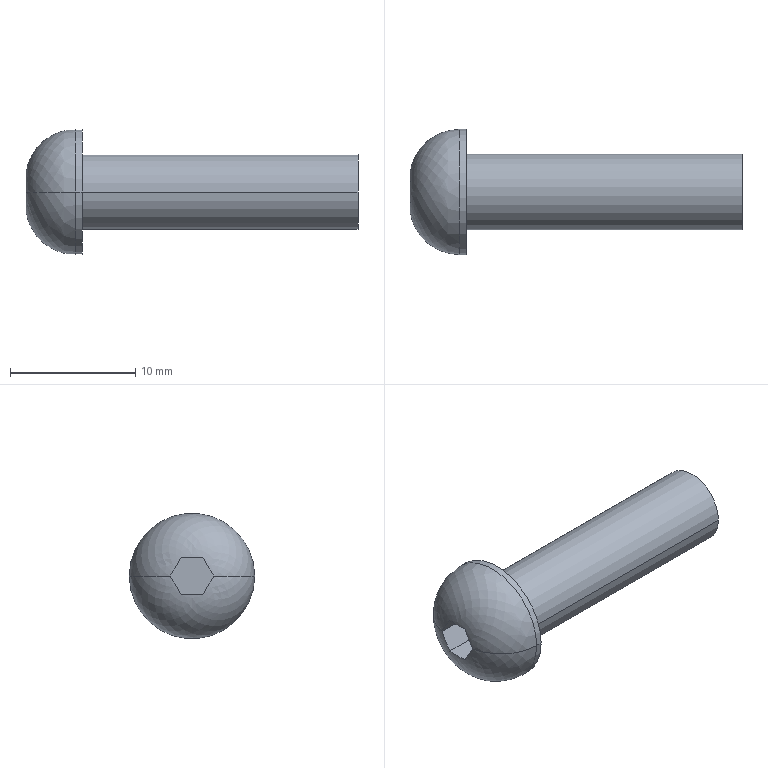Part | STEP file | Standoff screw φ6x12(M5) | 1 solid | 15 faces | box 26.469 x 10 x 10 mm | volume 868.238 mm3 | plane 9 | cylinder 4 | other 2 | commonest cylinder face diameters 6 x2 10 x2
STEP:
#1=CARTESIAN_POINT('',(0.,0.,0.));
#2=DIRECTION('',(0.,0.,1.));
#3=DIRECTION('',(1.,0.,0.));
#4=AXIS2_PLACEMENT_3D('',#1,#2,#3);
#5=CARTESIAN_POINT('',(4.5,3.,0.));
#6=VERTEX_POINT('',#5);
#7=CARTESIAN_POINT('',(4.5,-3.,0.));
#8=VERTEX_POINT('',#7);
#9=CARTESIAN_POINT('',(4.5,0.,0.));
#10=DIRECTION('',(1.,0.,0.));
#11=DIRECTION('',(0.,1.,0.));
#12=AXIS2_PLACEMENT_3D('',#9,#10,#11);
#13=CIRCLE('',#12,3.);
#14=CARTESIAN_POINT('',(26.5,0.,0.));
#15=DIRECTION('',(1.,0.,0.));
#16=DIRECTION('',(0.,1.,0.));
#17=AXIS2_PLACEMENT_3D('',#14,#15,#16);
#18=CYLINDRICAL_SURFACE('',#17,3.);
#19=CARTESIAN_POINT('',(0.,-22.));
#20=DIRECTION('',(1.,0.));
#21=VECTOR('',#20,1.);
#22=LINE('',#19,#21);
#23=(GEOMETRIC_REPRESENTATION_CONTEXT(2)PARAMETRIC_REPRESENTATION_CONTEXT()REPRESENTATION_CONTEXT('',''));
#24=DEFINITIONAL_REPRESENTATION('',(#22),#23);
#25=PCURVE('',#18,#24);
#26=CARTESIAN_POINT('',(4.5,-5.,0.));
#27=DIRECTION('',(-1.,0.,0.));
#28=DIRECTION('',(0.,-1.,0.));
#29=AXIS2_PLACEMENT_3D('',#26,#27,#28);
#30=PLANE('',#29);
#31=CARTESIAN_POINT('',(-8.,0.));
#32=CARTESIAN_POINT('',(-8.,5.196));
#33=CARTESIAN_POINT('',(-3.5,2.598));
#34=CARTESIAN_POINT('',(1.,0.));
#35=CARTESIAN_POINT('',(-3.5,-2.598));
#36=CARTESIAN_POINT('',(-8.,-5.196));
#37=CARTESIAN_POINT('',(-8.,0.));
#38=(BOUNDED_CURVE()B_SPLINE_CURVE(2,(#31,#32,#33,#34,#35,#36,#37),.UNSPECIFIED.,.T.,.F.)B_SPLINE_CURVE_WITH_KNOTS((1,2,2,2,2,1),(-2.094,0.,2.094,4.189,6.283,8.378),.UNSPECIFIED.)CURVE()GEOMETRIC_REPRESENTATION_ITEM()RATIONAL_B_SPLINE_CURVE((1.,0.5,1.,0.5,1.,0.5,1.))REPRESENTATION_ITEM(''));
#39=(GEOMETRIC_REPRESENTATION_CONTEXT(2)PARAMETRIC_REPRESENTATION_CONTEXT()REPRESENTATION_CONTEXT('',''));
#40=DEFINITIONAL_REPRESENTATION('',(#38),#39);
#41=PCURVE('',#30,#40);
#42=SURFACE_CURVE('',#13,(#25,#41),.PCURVE_S1.);
#43=EDGE_CURVE('',#6,#8,#42,.T.);
#44=ORIENTED_EDGE('',*,*,#43,.T.);
#45=CARTESIAN_POINT('',(26.5,-3.,0.));
#46=VERTEX_POINT('',#45);
#47=CARTESIAN_POINT('',(26.5,-3.,0.));
#48=DIRECTION('',(1.,0.,0.));
#49=VECTOR('',#48,1.);
#50=LINE('',#47,#49);
#51=CARTESIAN_POINT('',(3.142,0.));
#52=DIRECTION('',(0.,1.));
#53=VECTOR('',#52,1.);
#54=LINE('',#51,#53);
#55=(GEOMETRIC_REPRESENTATION_CONTEXT(2)PARAMETRIC_REPRESENTATION_CONTEXT()REPRESENTATION_CONTEXT('',''));
#56=DEFINITIONAL_REPRESENTATION('',(#54),#55);
#57=PCURVE('',#18,#56);
#58=CARTESIAN_POINT('',(26.5,0.,0.));
#59=DIRECTION('',(1.,0.,0.));
#60=DIRECTION('',(0.,1.,0.));
#61=AXIS2_PLACEMENT_3D('',#58,#59,#60);
#62=CYLINDRICAL_SURFACE('',#61,3.);
#63=CARTESIAN_POINT('',(3.142,0.));
#64=DIRECTION('',(0.,1.));
#65=VECTOR('',#64,1.);
#66=LINE('',#63,#65);
#67=(GEOMETRIC_REPRESENTATION_CONTEXT(2)PARAMETRIC_REPRESENTATION_CONTEXT()REPRESENTATION_CONTEXT('',''));
#68=DEFINITIONAL_REPRESENTATION('',(#66),#67);
#69=PCURVE('',#62,#68);
#70=SURFACE_CURVE('',#50,(#57,#69),.PCURVE_S1.);
#71=EDGE_CURVE('',#8,#46,#70,.T.);
#72=ORIENTED_EDGE('',*,*,#71,.T.);
#73=CARTESIAN_POINT('',(26.5,3.,0.));
#74=VERTEX_POINT('',#73);
#75=CARTESIAN_POINT('',(26.5,0.,0.));
#76=DIRECTION('',(1.,0.,0.));
#77=DIRECTION('',(0.,1.,0.));
#78=AXIS2_PLACEMENT_3D('',#75,#76,#77);
#79=CIRCLE('',#78,3.);
#80=CARTESIAN_POINT('',(0.,0.));
#81=DIRECTION('',(1.,0.));
#82=VECTOR('',#81,1.);
#83=LINE('',#80,#82);
#84=(GEOMETRIC_REPRESENTATION_CONTEXT(2)PARAMETRIC_REPRESENTATION_CONTEXT()REPRESENTATION_CONTEXT('',''));
#85=DEFINITIONAL_REPRESENTATION('',(#83),#84);
#86=PCURVE('',#18,#85);
#87=CARTESIAN_POINT('',(26.5,-3.,0.));
#88=DIRECTION('',(-1.,0.,0.));
#89=DIRECTION('',(0.,-1.,0.));
#90=AXIS2_PLACEMENT_3D('',#87,#88,#89);
#91=PLANE('',#90);
#92=CARTESIAN_POINT('',(-6.,0.));
#93=CARTESIAN_POINT('',(-6.,5.196));
#94=CARTESIAN_POINT('',(-1.5,2.598));
#95=CARTESIAN_POINT('',(3.,0.));
#96=CARTESIAN_POINT('',(-1.5,-2.598));
#97=CARTESIAN_POINT('',(-6.,-5.196));
#98=CARTESIAN_POINT('',(-6.,0.));
#99=(BOUNDED_CURVE()B_SPLINE_CURVE(2,(#92,#93,#94,#95,#96,#97,#98),.UNSPECIFIED.,.T.,.F.)B_SPLINE_CURVE_WITH_KNOTS((1,2,2,2,2,1),(-2.094,0.,2.094,4.189,6.283,8.378),.UNSPECIFIED.)CURVE()GEOMETRIC_REPRESENTATION_ITEM()RATIONAL_B_SPLINE_CURVE((1.,0.5,1.,0.5,1.,0.5,1.))REPRESENTATION_ITEM(''));
#100=(GEOMETRIC_REPRESENTATION_CONTEXT(2)PARAMETRIC_REPRESENTATION_CONTEXT()REPRESENTATION_CONTEXT('',''));
#101=DEFINITIONAL_REPRESENTATION('',(#99),#100);
#102=PCURVE('',#91,#101);
#103=SURFACE_CURVE('',#79,(#86,#102),.PCURVE_S1.);
#104=EDGE_CURVE('',#74,#46,#103,.T.);
#105=ORIENTED_EDGE('',*,*,#104,.F.);
#106=CARTESIAN_POINT('',(26.5,3.,0.));
#107=DIRECTION('',(1.,0.,0.));
#108=VECTOR('',#107,1.);
#109=LINE('',#106,#108);
#110=CARTESIAN_POINT('',(0.,0.));
#111=DIRECTION('',(0.,1.));
#112=VECTOR('',#111,1.);
#113=LINE('',#110,#112);
#114=(GEOMETRIC_REPRESENTATION_CONTEXT(2)PARAMETRIC_REPRESENTATION_CONTEXT()REPRESENTATION_CONTEXT('',''));
#115=DEFINITIONAL_REPRESENTATION('',(#113),#114);
#116=PCURVE('',#18,#115);
#117=CARTESIAN_POINT('',(6.283,0.));
#118=DIRECTION('',(0.,1.));
#119=VECTOR('',#118,1.);
#120=LINE('',#117,#119);
#121=(GEOMETRIC_REPRESENTATION_CONTEXT(2)PARAMETRIC_REPRESENTATION_CONTEXT()REPRESENTATION_CONTEXT('',''));
#122=DEFINITIONAL_REPRESENTATION('',(#120),#121);
#123=PCURVE('',#62,#122);
#124=SURFACE_CURVE('',#109,(#116,#123),.PCURVE_S1.);
#125=EDGE_CURVE('',#6,#74,#124,.T.);
#126=ORIENTED_EDGE('',*,*,#125,.F.);
#127=EDGE_LOOP('',(#44,#72,#105,#126));
#128=FACE_BOUND('',#127,.T.);
#129=ADVANCED_FACE('',(#128),#18,.T.);
#130=CARTESIAN_POINT('',(4.,5.,0.));
#131=VERTEX_POINT('',#130);
#132=CARTESIAN_POINT('',(4.,-5.,0.));
#133=VERTEX_POINT('',#132);
#134=CARTESIAN_POINT('',(4.,0.,0.));
#135=DIRECTION('',(1.,0.,0.));
#136=DIRECTION('',(0.,1.,0.));
#137=AXIS2_PLACEMENT_3D('',#134,#135,#136);
#138=CIRCLE('',#137,5.);
#139=CARTESIAN_POINT('',(26.5,0.,0.));
#140=DIRECTION('',(1.,0.,0.));
#141=DIRECTION('',(0.,1.,0.));
#142=AXIS2_PLACEMENT_3D('',#139,#140,#141);
#143=CYLINDRICAL_SURFACE('',#142,5.);
#144=CARTESIAN_POINT('',(0.,-22.5));
#145=DIRECTION('',(1.,0.));
#146=VECTOR('',#145,1.);
#147=LINE('',#144,#146);
#148=(GEOMETRIC_REPRESENTATION_CONTEXT(2)PARAMETRIC_REPRESENTATION_CONTEXT()REPRESENTATION_CONTEXT('',''));
#149=DEFINITIONAL_REPRESENTATION('',(#147),#148);
#150=PCURVE('',#143,#149);
#151=CARTESIAN_POINT('',(0.03137,1.5,0.));
#152=CARTESIAN_POINT('',(0.0916,1.978,0.));
#153=CARTESIAN_POINT('',(0.2209,2.447,0.));
#154=CARTESIAN_POINT('',(0.4178,2.896,0.));
#155=CARTESIAN_POINT('',(0.6776,3.31,0.));
#156=CARTESIAN_POINT('',(0.9929,3.681,0.));
#157=CARTESIAN_POINT('',(1.716,4.319,0.));
#158=CARTESIAN_POINT('',(2.123,4.585,0.));
#159=CARTESIAN_POINT('',(2.567,4.791,0.));
#160=CARTESIAN_POINT('',(3.036,4.93,0.));
#161=CARTESIAN_POINT('',(3.518,5.,0.));
#162=CARTESIAN_POINT('',(4.,5.,0.));
#163=B_SPLINE_CURVE_WITH_KNOTS('',6,(#151,#152,#153,#154,#155,#156,#157,#158,#159,#160,#161,#162),.UNSPECIFIED.,.F.,.F.,(7,5,7),(4.838,5.56,6.283),.UNSPECIFIED.);
#164=CARTESIAN_POINT('',(4.,0.,0.));
#165=DIRECTION('',(1.,0.,0.));
#166=AXIS1_PLACEMENT('',#164,#165);
#167=SURFACE_OF_REVOLUTION('',#163,#166);
#168=CARTESIAN_POINT('',(0.,6.283));
#169=DIRECTION('',(1.,0.));
#170=VECTOR('',#169,1.);
#171=LINE('',#168,#170);
#172=(GEOMETRIC_REPRESENTATION_CONTEXT(2)PARAMETRIC_REPRESENTATION_CONTEXT()REPRESENTATION_CONTEXT('',''));
#173=DEFINITIONAL_REPRESENTATION('',(#171),#172);
#174=PCURVE('',#167,#173);
#175=SURFACE_CURVE('',#138,(#150,#174),.PCURVE_S1.);
#176=EDGE_CURVE('',#131,#133,#175,.T.);
#177=ORIENTED_EDGE('',*,*,#176,.T.);
#178=CARTESIAN_POINT('',(4.5,-5.,0.));
#179=VERTEX_POINT('',#178);
#180=CARTESIAN_POINT('',(26.5,-5.,0.));
#181=DIRECTION('',(1.,0.,0.));
#182=VECTOR('',#181,1.);
#183=LINE('',#180,#182);
#184=CARTESIAN_POINT('',(3.142,0.));
#185=DIRECTION('',(0.,1.));
#186=VECTOR('',#185,1.);
#187=LINE('',#184,#186);
#188=(GEOMETRIC_REPRESENTATION_CONTEXT(2)PARAMETRIC_REPRESENTATION_CONTEXT()REPRESENTATION_CONTEXT('',''));
#189=DEFINITIONAL_REPRESENTATION('',(#187),#188);
#190=PCURVE('',#143,#189);
#191=CARTESIAN_POINT('',(26.5,0.,0.));
#192=DIRECTION('',(1.,0.,0.));
#193=DIRECTION('',(0.,1.,0.));
#194=AXIS2_PLACEMENT_3D('',#191,#192,#193);
#195=CYLINDRICAL_SURFACE('',#194,5.);
#196=CARTESIAN_POINT('',(3.142,0.));
#197=DIRECTION('',(0.,1.));
#198=VECTOR('',#197,1.);
#199=LINE('',#196,#198);
#200=(GEOMETRIC_REPRESENTATION_CONTEXT(2)PARAMETRIC_REPRESENTATION_CONTEXT()REPRESENTATION_CONTEXT('',''));
#201=DEFINITIONAL_REPRESENTATION('',(#199),#200);
#202=PCURVE('',#195,#201);
#203=SURFACE_CURVE('',#183,(#190,#202),.PCURVE_S1.);
#204=EDGE_CURVE('',#133,#179,#203,.T.);
#205=ORIENTED_EDGE('',*,*,#204,.T.);
#206=CARTESIAN_POINT('',(4.5,5.,0.));
#207=VERTEX_POINT('',#206);
#208=CARTESIAN_POINT('',(4.5,0.,0.));
#209=DIRECTION('',(1.,0.,0.));
#210=DIRECTION('',(0.,1.,0.));
#211=AXIS2_PLACEMENT_3D('',#208,#209,#210);
#212=CIRCLE('',#211,5.);
#213=CARTESIAN_POINT('',(0.,-22.));
#214=DIRECTION('',(1.,0.));
#215=VECTOR('',#214,1.);
#216=LINE('',#213,#215);
#217=(GEOMETRIC_REPRESENTATION_CONTEXT(2)PARAMETRIC_REPRESENTATION_CONTEXT()REPRESENTATION_CONTEXT('',''));
#218=DEFINITIONAL_REPRESENTATION('',(#216),#217);
#219=PCURVE('',#143,#218);
#220=CARTESIAN_POINT('',(-10.,0.));
#221=CARTESIAN_POINT('',(-10.,8.66));
#222=CARTESIAN_POINT('',(-2.5,4.33));
#223=CARTESIAN_POINT('',(5.,0.));
#224=CARTESIAN_POINT('',(-2.5,-4.33));
#225=CARTESIAN_POINT('',(-10.,-8.66));
#226=CARTESIAN_POINT('',(-10.,0.));
#227=(BOUNDED_CURVE()B_SPLINE_CURVE(2,(#220,#221,#222,#223,#224,#225,#226),.UNSPECIFIED.,.T.,.F.)B_SPLINE_CURVE_WITH_KNOTS((1,2,2,2,2,1),(-2.094,0.,2.094,4.189,6.283,8.378),.UNSPECIFIED.)CURVE()GEOMETRIC_REPRESENTATION_ITEM()RATIONAL_B_SPLINE_CURVE((1.,0.5,1.,0.5,1.,0.5,1.))REPRESENTATION_ITEM(''));
#228=(GEOMETRIC_REPRESENTATION_CONTEXT(2)PARAMETRIC_REPRESENTATION_CONTEXT()REPRESENTATION_CONTEXT('',''));
#229=DEFINITIONAL_REPRESENTATION('',(#227),#228);
#230=PCURVE('',#30,#229);
#231=SURFACE_CURVE('',#212,(#219,#230),.PCURVE_S1.);
#232=EDGE_CURVE('',#207,#179,#231,.T.);
#233=ORIENTED_EDGE('',*,*,#232,.F.);
#234=CARTESIAN_POINT('',(26.5,5.,0.));
#235=DIRECTION('',(1.,0.,0.));
#236=VECTOR('',#235,1.);
#237=LINE('',#234,#236);
#238=CARTESIAN_POINT('',(0.,0.));
#239=DIRECTION('',(0.,1.));
#240=VECTOR('',#239,1.);
#241=LINE('',#238,#240);
#242=(GEOMETRIC_REPRESENTATION_CONTEXT(2)PARAMETRIC_REPRESENTATION_CONTEXT()REPRESENTATION_CONTEXT('',''));
#243=DEFINITIONAL_REPRESENTATION('',(#241),#242);
#244=PCURVE('',#143,#243);
#245=CARTESIAN_POINT('',(6.283,0.));
#246=DIRECTION('',(0.,1.));
#247=VECTOR('',#246,1.);
#248=LINE('',#245,#247);
#249=(GEOMETRIC_REPRESENTATION_CONTEXT(2)PARAMETRIC_REPRESENTATION_CONTEXT()REPRESENTATION_CONTEXT('',''));
#250=DEFINITIONAL_REPRESENTATION('',(#248),#249);
#251=PCURVE('',#195,#250);
#252=SURFACE_CURVE('',#237,(#244,#251),.PCURVE_S1.);
#253=EDGE_CURVE('',#131,#207,#252,.T.);
#254=ORIENTED_EDGE('',*,*,#253,.F.);
#255=EDGE_LOOP('',(#177,#205,#233,#254));
#256=FACE_BOUND('',#255,.T.);
#257=ADVANCED_FACE('',(#256),#143,.T.);
#258=CARTESIAN_POINT('',(0.06756,-0.866,1.5));
#259=VERTEX_POINT('',#258);
#260=CARTESIAN_POINT('',(0.06756,-1.732,0.));
#261=VERTEX_POINT('',#260);
#262=CARTESIAN_POINT('',(0.06756,-0.866,1.5));
#263=CARTESIAN_POINT('',(0.04069,-1.01,1.25));
#264=CARTESIAN_POINT('',(0.02206,-1.299,0.75));
#265=CARTESIAN_POINT('',(0.04069,-1.588,0.25));
#266=CARTESIAN_POINT('',(0.06756,-1.732,0.));
#267=B_SPLINE_CURVE_WITH_KNOTS('',3,(#262,#263,#264,#265,#266),.UNSPECIFIED.,.F.,.F.,(4,1,4),(0.000000231,0.0008663,0.001732),.UNSPECIFIED.);
#268=CARTESIAN_POINT('',(2.094,4.896));
#269=CARTESIAN_POINT('',(2.108,4.893));
#270=CARTESIAN_POINT('',(2.134,4.887));
#271=CARTESIAN_POINT('',(2.176,4.878));
#272=CARTESIAN_POINT('',(2.22,4.87));
#273=CARTESIAN_POINT('',(2.266,4.862));
#274=CARTESIAN_POINT('',(2.313,4.856));
#275=CARTESIAN_POINT('',(2.361,4.85));
#276=CARTESIAN_POINT('',(2.411,4.846));
#277=CARTESIAN_POINT('',(2.462,4.842));
#278=CARTESIAN_POINT('',(2.513,4.84));
#279=CARTESIAN_POINT('',(2.566,4.838));
#280=CARTESIAN_POINT('',(2.618,4.838));
#281=CARTESIAN_POINT('',(2.67,4.838));
#282=CARTESIAN_POINT('',(2.723,4.84));
#283=CARTESIAN_POINT('',(2.774,4.842));
#284=CARTESIAN_POINT('',(2.825,4.846));
#285=CARTESIAN_POINT('',(2.875,4.85));
#286=CARTESIAN_POINT('',(2.923,4.856));
#287=CARTESIAN_POINT('',(2.97,4.862));
#288=CARTESIAN_POINT('',(3.016,4.87));
#289=CARTESIAN_POINT('',(3.06,4.878));
#290=CARTESIAN_POINT('',(3.102,4.887));
#291=CARTESIAN_POINT('',(3.128,4.893));
#292=CARTESIAN_POINT('',(3.142,4.896));
#293=B_SPLINE_CURVE_WITH_KNOTS('',3,(#268,#269,#270,#271,#272,#273,#274,#275,#276,#277,#278,#279,#280,#281,#282,#283,#284,#285,#286,#287,#288,#289,#290,#291,#292),.UNSPECIFIED.,.F.,.F.,(4,1,1,1,1,1,1,1,1,1,1,1,1,1,1,1,1,1,1,1,1,1,4),(0.000000231,0.00007896,0.0001577,0.0002364,0.0003151,0.0003939,0.0004726,0.0005513,0.0006301,0.0007088,0.0007875,0.0008663,0.000945,0.001024,0.001102,0.001181,0.00126,0.001339,0.001417,0.001496,0.001575,0.001654,0.001732),.QUASI_UNIFORM_KNOTS.);
#294=(GEOMETRIC_REPRESENTATION_CONTEXT(2)PARAMETRIC_REPRESENTATION_CONTEXT()REPRESENTATION_CONTEXT('',''));
#295=DEFINITIONAL_REPRESENTATION('',(#293),#294);
#296=PCURVE('',#167,#295);
#297=CARTESIAN_POINT('',(2.4,-1.732,0.));
#298=DIRECTION('',(0.,-0.866,0.5));
#299=DIRECTION('',(0.,-0.5,-0.866));
#300=AXIS2_PLACEMENT_3D('',#297,#298,#299);
#301=PLANE('',#300);
#302=CARTESIAN_POINT('',(-1.732,-2.332));
#303=CARTESIAN_POINT('',(-1.443,-2.359));
#304=CARTESIAN_POINT('',(-0.866,-2.378));
#305=CARTESIAN_POINT('',(-0.2887,-2.359));
#306=CARTESIAN_POINT('',(0.,-2.332));
#307=B_SPLINE_CURVE_WITH_KNOTS('',3,(#302,#303,#304,#305,#306),.UNSPECIFIED.,.F.,.F.,(4,1,4),(0.000000231,0.0008663,0.001732),.UNSPECIFIED.);
#308=(GEOMETRIC_REPRESENTATION_CONTEXT(2)PARAMETRIC_REPRESENTATION_CONTEXT()REPRESENTATION_CONTEXT('',''));
#309=DEFINITIONAL_REPRESENTATION('',(#307),#308);
#310=PCURVE('',#301,#309);
#311=SURFACE_CURVE('',#267,(#296,#310),.PCURVE_S1.);
#312=EDGE_CURVE('',#259,#261,#311,.T.);
#313=ORIENTED_EDGE('',*,*,#312,.T.);
#314=CARTESIAN_POINT('',(4.,-1.,0.));
#315=DIRECTION('',(0.,0.,1.));
#316=DIRECTION('',(0.,-1.,0.));
#317=AXIS2_PLACEMENT_3D('',#314,#315,#316);
#318=CIRCLE('',#317,4.);
#319=CARTESIAN_POINT('',(3.142,0.));
#320=DIRECTION('',(0.,1.));
#321=VECTOR('',#320,1.);
#322=LINE('',#319,#321);
#323=(GEOMETRIC_REPRESENTATION_CONTEXT(2)PARAMETRIC_REPRESENTATION_CONTEXT()REPRESENTATION_CONTEXT('',''));
#324=DEFINITIONAL_REPRESENTATION('',(#322),#323);
#325=PCURVE('',#167,#324);
#326=CARTESIAN_POINT('',(0.03137,1.5,0.));
#327=CARTESIAN_POINT('',(0.0916,1.978,0.));
#328=CARTESIAN_POINT('',(0.2209,2.447,0.));
#329=CARTESIAN_POINT('',(0.4178,2.896,0.));
#330=CARTESIAN_POINT('',(0.6776,3.31,0.));
#331=CARTESIAN_POINT('',(0.9929,3.681,0.));
#332=CARTESIAN_POINT('',(1.716,4.319,0.));
#333=CARTESIAN_POINT('',(2.123,4.585,0.));
#334=CARTESIAN_POINT('',(2.567,4.791,0.));
#335=CARTESIAN_POINT('',(3.036,4.93,0.));
#336=CARTESIAN_POINT('',(3.518,5.,0.));
#337=CARTESIAN_POINT('',(4.,5.,0.));
#338=B_SPLINE_CURVE_WITH_KNOTS('',6,(#326,#327,#328,#329,#330,#331,#332,#333,#334,#335,#336,#337),.UNSPECIFIED.,.F.,.F.,(7,5,7),(4.838,5.56,6.283),.UNSPECIFIED.);
#339=CARTESIAN_POINT('',(4.,0.,0.));
#340=DIRECTION('',(1.,0.,0.));
#341=AXIS1_PLACEMENT('',#339,#340);
#342=SURFACE_OF_REVOLUTION('',#338,#341);
#343=CARTESIAN_POINT('',(3.142,0.));
#344=DIRECTION('',(0.,1.));
#345=VECTOR('',#344,1.);
#346=LINE('',#343,#345);
#347=(GEOMETRIC_REPRESENTATION_CONTEXT(2)PARAMETRIC_REPRESENTATION_CONTEXT()REPRESENTATION_CONTEXT('',''));
#348=DEFINITIONAL_REPRESENTATION('',(#346),#347);
#349=PCURVE('',#342,#348);
#350=SURFACE_CURVE('',#318,(#325,#349),.PCURVE_S1.);
#351=EDGE_CURVE('',#261,#133,#350,.T.);
#352=ORIENTED_EDGE('',*,*,#351,.T.);
#353=ORIENTED_EDGE('',*,*,#176,.F.);
#354=CARTESIAN_POINT('',(0.06756,1.732,0.));
#355=VERTEX_POINT('',#354);
#356=CARTESIAN_POINT('',(4.,1.,0.));
#357=DIRECTION('',(0.,0.,-1.));
#358=DIRECTION('',(-1.,0.,0.));
#359=AXIS2_PLACEMENT_3D('',#356,#357,#358);
#360=CIRCLE('',#359,4.);
#361=CARTESIAN_POINT('',(0.,4.712));
#362=DIRECTION('',(0.,1.));
#363=VECTOR('',#362,1.);
#364=LINE('',#361,#363);
#365=(GEOMETRIC_REPRESENTATION_CONTEXT(2)PARAMETRIC_REPRESENTATION_CONTEXT()REPRESENTATION_CONTEXT('',''));
#366=DEFINITIONAL_REPRESENTATION('',(#364),#365);
#367=PCURVE('',#167,#366);
#368=CARTESIAN_POINT('',(6.283,4.712));
#369=DIRECTION('',(0.,1.));
#370=VECTOR('',#369,1.);
#371=LINE('',#368,#370);
#372=(GEOMETRIC_REPRESENTATION_CONTEXT(2)PARAMETRIC_REPRESENTATION_CONTEXT()REPRESENTATION_CONTEXT('',''));
#373=DEFINITIONAL_REPRESENTATION('',(#371),#372);
#374=PCURVE('',#342,#373);
#375=SURFACE_CURVE('',#360,(#367,#374),.PCURVE_S1.);
#376=EDGE_CURVE('',#355,#131,#375,.T.);
#377=ORIENTED_EDGE('',*,*,#376,.F.);
#378=CARTESIAN_POINT('',(0.06756,0.866,1.5));
#379=VERTEX_POINT('',#378);
#380=CARTESIAN_POINT('',(0.06756,1.732,0.));
#381=CARTESIAN_POINT('',(0.04069,1.588,0.25));
#382=CARTESIAN_POINT('',(0.02206,1.299,0.75));
#383=CARTESIAN_POINT('',(0.04069,1.01,1.25));
#384=CARTESIAN_POINT('',(0.06756,0.866,1.5));
#385=B_SPLINE_CURVE_WITH_KNOTS('',3,(#380,#381,#382,#383,#384),.UNSPECIFIED.,.F.,.F.,(4,1,4),(0.000000231,0.0008663,0.001732),.QUASI_UNIFORM_KNOTS.);
#386=CARTESIAN_POINT('',(0.,4.896));
#387=CARTESIAN_POINT('',(0.01312,4.893));
#388=CARTESIAN_POINT('',(0.03996,4.887));
#389=CARTESIAN_POINT('',(0.082,4.878));
#390=CARTESIAN_POINT('',(0.1258,4.87));
#391=CARTESIAN_POINT('',(0.1712,4.862));
#392=CARTESIAN_POINT('',(0.2183,4.856));
#393=CARTESIAN_POINT('',(0.2667,4.85));
#394=CARTESIAN_POINT('',(0.3165,4.846));
#395=CARTESIAN_POINT('',(0.3673,4.842));
#396=CARTESIAN_POINT('',(0.4189,4.84));
#397=CARTESIAN_POINT('',(0.4711,4.838));
#398=CARTESIAN_POINT('',(0.5236,4.838));
#399=CARTESIAN_POINT('',(0.5761,4.838));
#400=CARTESIAN_POINT('',(0.6283,4.84));
#401=CARTESIAN_POINT('',(0.6799,4.842));
#402=CARTESIAN_POINT('',(0.7307,4.846));
#403=CARTESIAN_POINT('',(0.7805,4.85));
#404=CARTESIAN_POINT('',(0.8289,4.856));
#405=CARTESIAN_POINT('',(0.876,4.862));
#406=CARTESIAN_POINT('',(0.9214,4.87));
#407=CARTESIAN_POINT('',(0.9652,4.878));
#408=CARTESIAN_POINT('',(1.007,4.887));
#409=CARTESIAN_POINT('',(1.034,4.893));
#410=CARTESIAN_POINT('',(1.047,4.896));
#411=B_SPLINE_CURVE_WITH_KNOTS('',3,(#386,#387,#388,#389,#390,#391,#392,#393,#394,#395,#396,#397,#398,#399,#400,#401,#402,#403,#404,#405,#406,#407,#408,#409,#410),.UNSPECIFIED.,.F.,.F.,(4,1,1,1,1,1,1,1,1,1,1,1,1,1,1,1,1,1,1,1,1,1,4),(0.000000231,0.00007896,0.0001577,0.0002364,0.0003151,0.0003939,0.0004726,0.0005513,0.0006301,0.0007088,0.0007875,0.0008663,0.000945,0.001024,0.001102,0.001181,0.00126,0.001339,0.001417,0.001496,0.001575,0.001654,0.001732),.QUASI_UNIFORM_KNOTS.);
#412=(GEOMETRIC_REPRESENTATION_CONTEXT(2)PARAMETRIC_REPRESENTATION_CONTEXT()REPRESENTATION_CONTEXT('',''));
#413=DEFINITIONAL_REPRESENTATION('',(#411),#412);
#414=PCURVE('',#167,#413);
#415=CARTESIAN_POINT('',(2.4,0.866,1.5));
#416=DIRECTION('',(0.,0.866,0.5));
#417=DIRECTION('',(0.,-0.5,0.866));
#418=AXIS2_PLACEMENT_3D('',#415,#416,#417);
#419=PLANE('',#418);
#420=CARTESIAN_POINT('',(-1.732,-2.332));
#421=CARTESIAN_POINT('',(-1.443,-2.359));
#422=CARTESIAN_POINT('',(-0.866,-2.378));
#423=CARTESIAN_POINT('',(-0.2887,-2.359));
#424=CARTESIAN_POINT('',(0.,-2.332));
#425=B_SPLINE_CURVE_WITH_KNOTS('',3,(#420,#421,#422,#423,#424),.UNSPECIFIED.,.F.,.F.,(4,1,4),(0.000000231,0.0008663,0.001732),.QUASI_UNIFORM_KNOTS.);
#426=(GEOMETRIC_REPRESENTATION_CONTEXT(2)PARAMETRIC_REPRESENTATION_CONTEXT()REPRESENTATION_CONTEXT('',''));
#427=DEFINITIONAL_REPRESENTATION('',(#425),#426);
#428=PCURVE('',#419,#427);
#429=SURFACE_CURVE('',#385,(#414,#428),.PCURVE_S1.);
#430=EDGE_CURVE('',#355,#379,#429,.T.);
#431=ORIENTED_EDGE('',*,*,#430,.T.);
#432=CARTESIAN_POINT('',(0.06756,0.866,1.5));
#433=CARTESIAN_POINT('',(0.04093,0.5799,1.5));
#434=CARTESIAN_POINT('',(0.0314,0.2903,1.5));
#435=CARTESIAN_POINT('',(0.03134,-0.2878,1.5));
#436=CARTESIAN_POINT('',(0.04077,-0.5782,1.5));
#437=CARTESIAN_POINT('',(0.06756,-0.866,1.5));
#438=B_SPLINE_CURVE_WITH_KNOTS('',3,(#432,#433,#434,#435,#436,#437),.UNSPECIFIED.,.F.,.F.,(4,2,4),(0.0271,0.02797,0.02884),.UNSPECIFIED.);
#439=CARTESIAN_POINT('',(1.047,4.896));
#440=CARTESIAN_POINT('',(1.06,4.893));
#441=CARTESIAN_POINT('',(1.087,4.887));
#442=CARTESIAN_POINT('',(1.129,4.878));
#443=CARTESIAN_POINT('',(1.172,4.87));
#444=CARTESIAN_POINT('',(1.217,4.862));
#445=CARTESIAN_POINT('',(1.264,4.856));
#446=CARTESIAN_POINT('',(1.313,4.85));
#447=CARTESIAN_POINT('',(1.363,4.846));
#448=CARTESIAN_POINT('',(1.413,4.842));
#449=CARTESIAN_POINT('',(1.465,4.84));
#450=CARTESIAN_POINT('',(1.517,4.838));
#451=CARTESIAN_POINT('',(1.57,4.838));
#452=CARTESIAN_POINT('',(1.623,4.838));
#453=CARTESIAN_POINT('',(1.675,4.84));
#454=CARTESIAN_POINT('',(1.727,4.842));
#455=CARTESIAN_POINT('',(1.778,4.846));
#456=CARTESIAN_POINT('',(1.827,4.85));
#457=CARTESIAN_POINT('',(1.876,4.856));
#458=CARTESIAN_POINT('',(1.923,4.862));
#459=CARTESIAN_POINT('',(1.969,4.87));
#460=CARTESIAN_POINT('',(2.013,4.878));
#461=CARTESIAN_POINT('',(2.055,4.887));
#462=CARTESIAN_POINT('',(2.081,4.893));
#463=CARTESIAN_POINT('',(2.094,4.896));
#464=B_SPLINE_CURVE_WITH_KNOTS('',3,(#439,#440,#441,#442,#443,#444,#445,#446,#447,#448,#449,#450,#451,#452,#453,#454,#455,#456,#457,#458,#459,#460,#461,#462,#463),.UNSPECIFIED.,.F.,.F.,(4,1,1,1,1,1,1,1,1,1,1,1,1,1,1,1,1,1,1,1,1,1,4),(0.0271,0.02718,0.02726,0.02734,0.02742,0.0275,0.02758,0.02765,0.02773,0.02781,0.02789,0.02797,0.02805,0.02813,0.02821,0.02828,0.02836,0.02844,0.02852,0.0286,0.02868,0.02876,0.02884),.QUASI_UNIFORM_KNOTS.);
#465=(GEOMETRIC_REPRESENTATION_CONTEXT(2)PARAMETRIC_REPRESENTATION_CONTEXT()REPRESENTATION_CONTEXT('',''));
#466=DEFINITIONAL_REPRESENTATION('',(#464),#465);
#467=PCURVE('',#167,#466);
#468=CARTESIAN_POINT('',(2.4,-0.866,1.5));
#469=DIRECTION('',(0.,0.,1.));
#470=DIRECTION('',(0.,-1.,0.));
#471=AXIS2_PLACEMENT_3D('',#468,#469,#470);
#472=PLANE('',#471);
#473=CARTESIAN_POINT('',(-1.732,-2.332));
#474=CARTESIAN_POINT('',(-1.446,-2.359));
#475=CARTESIAN_POINT('',(-1.156,-2.369));
#476=CARTESIAN_POINT('',(-0.5782,-2.369));
#477=CARTESIAN_POINT('',(-0.2878,-2.359));
#478=CARTESIAN_POINT('',(0.,-2.332));
#479=B_SPLINE_CURVE_WITH_KNOTS('',3,(#473,#474,#475,#476,#477,#478),.UNSPECIFIED.,.F.,.F.,(4,2,4),(0.0271,0.02797,0.02884),.UNSPECIFIED.);
#480=(GEOMETRIC_REPRESENTATION_CONTEXT(2)PARAMETRIC_REPRESENTATION_CONTEXT()REPRESENTATION_CONTEXT('',''));
#481=DEFINITIONAL_REPRESENTATION('',(#479),#480);
#482=PCURVE('',#472,#481);
#483=SURFACE_CURVE('',#438,(#467,#482),.PCURVE_S1.);
#484=EDGE_CURVE('',#379,#259,#483,.T.);
#485=ORIENTED_EDGE('',*,*,#484,.T.);
#486=EDGE_LOOP('',(#313,#352,#353,#377,#431,#485));
#487=FACE_BOUND('',#486,.T.);
#488=ADVANCED_FACE('',(#487),#167,.T.);
#489=ORIENTED_EDGE('',*,*,#351,.F.);
#490=CARTESIAN_POINT('',(0.06756,-0.866,-1.5));
#491=VERTEX_POINT('',#490);
#492=CARTESIAN_POINT('',(0.06756,-1.732,0.));
#493=CARTESIAN_POINT('',(0.04069,-1.588,-0.25));
#494=CARTESIAN_POINT('',(0.02206,-1.299,-0.75));
#495=CARTESIAN_POINT('',(0.04069,-1.01,-1.25));
#496=CARTESIAN_POINT('',(0.06756,-0.866,-1.5));
#497=B_SPLINE_CURVE_WITH_KNOTS('',3,(#492,#493,#494,#495,#496),.UNSPECIFIED.,.F.,.F.,(4,1,4),(0.000000231,0.0008663,0.001732),.QUASI_UNIFORM_KNOTS.);
#498=CARTESIAN_POINT('',(3.142,4.896));
#499=CARTESIAN_POINT('',(3.155,4.893));
#500=CARTESIAN_POINT('',(3.182,4.887));
#501=CARTESIAN_POINT('',(3.224,4.878));
#502=CARTESIAN_POINT('',(3.267,4.87));
#503=CARTESIAN_POINT('',(3.313,4.862));
#504=CARTESIAN_POINT('',(3.36,4.856));
#505=CARTESIAN_POINT('',(3.408,4.85));
#506=CARTESIAN_POINT('',(3.458,4.846));
#507=CARTESIAN_POINT('',(3.509,4.842));
#508=CARTESIAN_POINT('',(3.561,4.84));
#509=CARTESIAN_POINT('',(3.613,4.838));
#510=CARTESIAN_POINT('',(3.665,4.838));
#511=CARTESIAN_POINT('',(3.718,4.838));
#512=CARTESIAN_POINT('',(3.77,4.84));
#513=CARTESIAN_POINT('',(3.822,4.842));
#514=CARTESIAN_POINT('',(3.872,4.846));
#515=CARTESIAN_POINT('',(3.922,4.85));
#516=CARTESIAN_POINT('',(3.971,4.856));
#517=CARTESIAN_POINT('',(4.018,4.862));
#518=CARTESIAN_POINT('',(4.063,4.87));
#519=CARTESIAN_POINT('',(4.107,4.878));
#520=CARTESIAN_POINT('',(4.149,4.887));
#521=CARTESIAN_POINT('',(4.176,4.893));
#522=CARTESIAN_POINT('',(4.189,4.896));
#523=B_SPLINE_CURVE_WITH_KNOTS('',3,(#498,#499,#500,#501,#502,#503,#504,#505,#506,#507,#508,#509,#510,#511,#512,#513,#514,#515,#516,#517,#518,#519,#520,#521,#522),.UNSPECIFIED.,.F.,.F.,(4,1,1,1,1,1,1,1,1,1,1,1,1,1,1,1,1,1,1,1,1,1,4),(0.000000231,0.00007896,0.0001577,0.0002364,0.0003151,0.0003939,0.0004726,0.0005513,0.0006301,0.0007088,0.0007875,0.0008663,0.000945,0.001024,0.001102,0.001181,0.00126,0.001339,0.001417,0.001496,0.001575,0.001654,0.001732),.QUASI_UNIFORM_KNOTS.);
#524=(GEOMETRIC_REPRESENTATION_CONTEXT(2)PARAMETRIC_REPRESENTATION_CONTEXT()REPRESENTATION_CONTEXT('',''));
#525=DEFINITIONAL_REPRESENTATION('',(#523),#524);
#526=PCURVE('',#342,#525);
#527=CARTESIAN_POINT('',(2.4,-0.866,-1.5));
#528=DIRECTION('',(0.,-0.866,-0.5));
#529=DIRECTION('',(0.,0.5,-0.866));
#530=AXIS2_PLACEMENT_3D('',#527,#528,#529);
#531=PLANE('',#530);
#532=CARTESIAN_POINT('',(-1.732,-2.332));
#533=CARTESIAN_POINT('',(-1.443,-2.359));
#534=CARTESIAN_POINT('',(-0.866,-2.378));
#535=CARTESIAN_POINT('',(-0.2887,-2.359));
#536=CARTESIAN_POINT('',(0.,-2.332));
#537=B_SPLINE_CURVE_WITH_KNOTS('',3,(#532,#533,#534,#535,#536),.UNSPECIFIED.,.F.,.F.,(4,1,4),(0.000000231,0.0008663,0.001732),.QUASI_UNIFORM_KNOTS.);
#538=(GEOMETRIC_REPRESENTATION_CONTEXT(2)PARAMETRIC_REPRESENTATION_CONTEXT()REPRESENTATION_CONTEXT('',''));
#539=DEFINITIONAL_REPRESENTATION('',(#537),#538);
#540=PCURVE('',#531,#539);
#541=SURFACE_CURVE('',#497,(#526,#540),.PCURVE_S1.);
#542=EDGE_CURVE('',#261,#491,#541,.T.);
#543=ORIENTED_EDGE('',*,*,#542,.T.);
#544=CARTESIAN_POINT('',(0.06756,0.866,-1.5));
#545=VERTEX_POINT('',#544);
#546=CARTESIAN_POINT('',(0.06756,-0.866,-1.5));
#547=CARTESIAN_POINT('',(0.04093,-0.5799,-1.5));
#548=CARTESIAN_POINT('',(0.0314,-0.2903,-1.5));
#549=CARTESIAN_POINT('',(0.03134,0.2878,-1.5));
#550=CARTESIAN_POINT('',(0.04077,0.5782,-1.5));
#551=CARTESIAN_POINT('',(0.06756,0.866,-1.5));
#552=B_SPLINE_CURVE_WITH_KNOTS('',3,(#546,#547,#548,#549,#550,#551),.UNSPECIFIED.,.F.,.F.,(4,2,4),(0.0271,0.02797,0.02884),.UNSPECIFIED.);
#553=CARTESIAN_POINT('',(4.189,4.896));
#554=CARTESIAN_POINT('',(4.202,4.893));
#555=CARTESIAN_POINT('',(4.228,4.887));
#556=CARTESIAN_POINT('',(4.27,4.878));
#557=CARTESIAN_POINT('',(4.314,4.87));
#558=CARTESIAN_POINT('',(4.359,4.862));
#559=CARTESIAN_POINT('',(4.406,4.856));
#560=CARTESIAN_POINT('',(4.454,4.85));
#561=CARTESIAN_POINT('',(4.504,4.846));
#562=CARTESIAN_POINT('',(4.555,4.842));
#563=CARTESIAN_POINT('',(4.607,4.84));
#564=CARTESIAN_POINT('',(4.659,4.838));
#565=CARTESIAN_POINT('',(4.712,4.838));
#566=CARTESIAN_POINT('',(4.764,4.838));
#567=CARTESIAN_POINT('',(4.816,4.84));
#568=CARTESIAN_POINT('',(4.868,4.842));
#569=CARTESIAN_POINT('',(4.919,4.846));
#570=CARTESIAN_POINT('',(4.969,4.85));
#571=CARTESIAN_POINT('',(5.018,4.856));
#572=CARTESIAN_POINT('',(5.065,4.862));
#573=CARTESIAN_POINT('',(5.11,4.87));
#574=CARTESIAN_POINT('',(5.154,4.878));
#575=CARTESIAN_POINT('',(5.196,4.887));
#576=CARTESIAN_POINT('',(5.223,4.893));
#577=CARTESIAN_POINT('',(5.236,4.896));
#578=B_SPLINE_CURVE_WITH_KNOTS('',3,(#553,#554,#555,#556,#557,#558,#559,#560,#561,#562,#563,#564,#565,#566,#567,#568,#569,#570,#571,#572,#573,#574,#575,#576,#577),.UNSPECIFIED.,.F.,.F.,(4,1,1,1,1,1,1,1,1,1,1,1,1,1,1,1,1,1,1,1,1,1,4),(0.0271,0.02718,0.02726,0.02734,0.02742,0.0275,0.02758,0.02765,0.02773,0.02781,0.02789,0.02797,0.02805,0.02813,0.02821,0.02828,0.02836,0.02844,0.02852,0.0286,0.02868,0.02876,0.02884),.QUASI_UNIFORM_KNOTS.);
#579=(GEOMETRIC_REPRESENTATION_CONTEXT(2)PARAMETRIC_REPRESENTATION_CONTEXT()REPRESENTATION_CONTEXT('',''));
#580=DEFINITIONAL_REPRESENTATION('',(#578),#579);
#581=PCURVE('',#342,#580);
#582=CARTESIAN_POINT('',(2.4,0.866,-1.5));
#583=DIRECTION('',(0.,0.,-1.));
#584=DIRECTION('',(-1.,0.,0.));
#585=AXIS2_PLACEMENT_3D('',#582,#583,#584);
#586=PLANE('',#585);
#587=CARTESIAN_POINT('',(2.332,-1.732));
#588=CARTESIAN_POINT('',(2.359,-1.446));
#589=CARTESIAN_POINT('',(2.369,-1.156));
#590=CARTESIAN_POINT('',(2.369,-0.5782));
#591=CARTESIAN_POINT('',(2.359,-0.2878));
#592=CARTESIAN_POINT('',(2.332,0.));
#593=B_SPLINE_CURVE_WITH_KNOTS('',3,(#587,#588,#589,#590,#591,#592),.UNSPECIFIED.,.F.,.F.,(4,2,4),(0.0271,0.02797,0.02884),.UNSPECIFIED.);
#594=(GEOMETRIC_REPRESENTATION_CONTEXT(2)PARAMETRIC_REPRESENTATION_CONTEXT()REPRESENTATION_CONTEXT('',''));
#595=DEFINITIONAL_REPRESENTATION('',(#593),#594);
#596=PCURVE('',#586,#595);
#597=SURFACE_CURVE('',#552,(#581,#596),.PCURVE_S1.);
#598=EDGE_CURVE('',#491,#545,#597,.T.);
#599=ORIENTED_EDGE('',*,*,#598,.T.);
#600=CARTESIAN_POINT('',(0.06756,0.866,-1.5));
#601=CARTESIAN_POINT('',(0.04069,1.01,-1.25));
#602=CARTESIAN_POINT('',(0.02206,1.299,-0.75));
#603=CARTESIAN_POINT('',(0.04069,1.588,-0.25));
#604=CARTESIAN_POINT('',(0.06756,1.732,0.));
#605=B_SPLINE_CURVE_WITH_KNOTS('',3,(#600,#601,#602,#603,#604),.UNSPECIFIED.,.F.,.F.,(4,1,4),(0.000000231,0.0008663,0.001732),.QUASI_UNIFORM_KNOTS.);
#606=CARTESIAN_POINT('',(5.236,4.896));
#607=CARTESIAN_POINT('',(5.249,4.893));
#608=CARTESIAN_POINT('',(5.276,4.887));
#609=CARTESIAN_POINT('',(5.318,4.878));
#610=CARTESIAN_POINT('',(5.362,4.87));
#611=CARTESIAN_POINT('',(5.407,4.862));
#612=CARTESIAN_POINT('',(5.454,4.856));
#613=CARTESIAN_POINT('',(5.503,4.85));
#614=CARTESIAN_POINT('',(5.552,4.846));
#615=CARTESIAN_POINT('',(5.603,4.842));
#616=CARTESIAN_POINT('',(5.655,4.84));
#617=CARTESIAN_POINT('',(5.707,4.838));
#618=CARTESIAN_POINT('',(5.76,4.838));
#619=CARTESIAN_POINT('',(5.812,4.838));
#620=CARTESIAN_POINT('',(5.864,4.84));
#621=CARTESIAN_POINT('',(5.916,4.842));
#622=CARTESIAN_POINT('',(5.967,4.846));
#623=CARTESIAN_POINT('',(6.016,4.85));
#624=CARTESIAN_POINT('',(6.065,4.856));
#625=CARTESIAN_POINT('',(6.112,4.862));
#626=CARTESIAN_POINT('',(6.157,4.87));
#627=CARTESIAN_POINT('',(6.201,4.878));
#628=CARTESIAN_POINT('',(6.243,4.887));
#629=CARTESIAN_POINT('',(6.27,4.893));
#630=CARTESIAN_POINT('',(6.283,4.896));
#631=B_SPLINE_CURVE_WITH_KNOTS('',3,(#606,#607,#608,#609,#610,#611,#612,#613,#614,#615,#616,#617,#618,#619,#620,#621,#622,#623,#624,#625,#626,#627,#628,#629,#630),.UNSPECIFIED.,.F.,.F.,(4,1,1,1,1,1,1,1,1,1,1,1,1,1,1,1,1,1,1,1,1,1,4),(0.000000231,0.00007896,0.0001577,0.0002364,0.0003151,0.0003939,0.0004726,0.0005513,0.0006301,0.0007088,0.0007875,0.0008663,0.000945,0.001024,0.001102,0.001181,0.00126,0.001339,0.001417,0.001496,0.001575,0.001654,0.001732),.QUASI_UNIFORM_KNOTS.);
#632=(GEOMETRIC_REPRESENTATION_CONTEXT(2)PARAMETRIC_REPRESENTATION_CONTEXT()REPRESENTATION_CONTEXT('',''));
#633=DEFINITIONAL_REPRESENTATION('',(#631),#632);
#634=PCURVE('',#342,#633);
#635=CARTESIAN_POINT('',(2.4,1.732,0.));
#636=DIRECTION('',(0.,0.866,-0.5));
#637=DIRECTION('',(0.,0.5,0.866));
#638=AXIS2_PLACEMENT_3D('',#635,#636,#637);
#639=PLANE('',#638);
#640=CARTESIAN_POINT('',(-1.732,-2.332));
#641=CARTESIAN_POINT('',(-1.443,-2.359));
#642=CARTESIAN_POINT('',(-0.866,-2.378));
#643=CARTESIAN_POINT('',(-0.2887,-2.359));
#644=CARTESIAN_POINT('',(0.,-2.332));
#645=B_SPLINE_CURVE_WITH_KNOTS('',3,(#640,#641,#642,#643,#644),.UNSPECIFIED.,.F.,.F.,(4,1,4),(0.000000231,0.0008663,0.001732),.QUASI_UNIFORM_KNOTS.);
#646=(GEOMETRIC_REPRESENTATION_CONTEXT(2)PARAMETRIC_REPRESENTATION_CONTEXT()REPRESENTATION_CONTEXT('',''));
#647=DEFINITIONAL_REPRESENTATION('',(#645),#646);
#648=PCURVE('',#639,#647);
#649=SURFACE_CURVE('',#605,(#634,#648),.PCURVE_S1.);
#650=EDGE_CURVE('',#545,#355,#649,.T.);
#651=ORIENTED_EDGE('',*,*,#650,.T.);
#652=ORIENTED_EDGE('',*,*,#376,.T.);
#653=CARTESIAN_POINT('',(4.,0.,0.));
#654=DIRECTION('',(1.,0.,0.));
#655=DIRECTION('',(0.,1.,0.));
#656=AXIS2_PLACEMENT_3D('',#653,#654,#655);
#657=CIRCLE('',#656,5.);
#658=CARTESIAN_POINT('',(0.,6.283));
#659=DIRECTION('',(1.,0.));
#660=VECTOR('',#659,1.);
#661=LINE('',#658,#660);
#662=(GEOMETRIC_REPRESENTATION_CONTEXT(2)PARAMETRIC_REPRESENTATION_CONTEXT()REPRESENTATION_CONTEXT('',''));
#663=DEFINITIONAL_REPRESENTATION('',(#661),#662);
#664=PCURVE('',#342,#663);
#665=CARTESIAN_POINT('',(0.,-22.5));
#666=DIRECTION('',(1.,0.));
#667=VECTOR('',#666,1.);
#668=LINE('',#665,#667);
#669=(GEOMETRIC_REPRESENTATION_CONTEXT(2)PARAMETRIC_REPRESENTATION_CONTEXT()REPRESENTATION_CONTEXT('',''));
#670=DEFINITIONAL_REPRESENTATION('',(#668),#669);
#671=PCURVE('',#195,#670);
#672=SURFACE_CURVE('',#657,(#664,#671),.PCURVE_S1.);
#673=EDGE_CURVE('',#133,#131,#672,.T.);
#674=ORIENTED_EDGE('',*,*,#673,.F.);
#675=EDGE_LOOP('',(#489,#543,#599,#651,#652,#674));
#676=FACE_BOUND('',#675,.T.);
#677=ADVANCED_FACE('',(#676),#342,.T.);
#678=ORIENTED_EDGE('',*,*,#204,.F.);
#679=ORIENTED_EDGE('',*,*,#673,.T.);
#680=ORIENTED_EDGE('',*,*,#253,.T.);
#681=CARTESIAN_POINT('',(4.5,0.,0.));
#682=DIRECTION('',(1.,0.,0.));
#683=DIRECTION('',(0.,1.,0.));
#684=AXIS2_PLACEMENT_3D('',#681,#682,#683);
#685=CIRCLE('',#684,5.);
#686=CARTESIAN_POINT('',(0.,-22.));
#687=DIRECTION('',(1.,0.));
#688=VECTOR('',#687,1.);
#689=LINE('',#686,#688);
#690=(GEOMETRIC_REPRESENTATION_CONTEXT(2)PARAMETRIC_REPRESENTATION_CONTEXT()REPRESENTATION_CONTEXT('',''));
#691=DEFINITIONAL_REPRESENTATION('',(#689),#690);
#692=PCURVE('',#195,#691);
#693=CARTESIAN_POINT('',(-10.,0.));
#694=CARTESIAN_POINT('',(-10.,8.66));
#695=CARTESIAN_POINT('',(-2.5,4.33));
#696=CARTESIAN_POINT('',(5.,0.));
#697=CARTESIAN_POINT('',(-2.5,-4.33));
#698=CARTESIAN_POINT('',(-10.,-8.66));
#699=CARTESIAN_POINT('',(-10.,0.));
#700=(BOUNDED_CURVE()B_SPLINE_CURVE(2,(#693,#694,#695,#696,#697,#698,#699),.UNSPECIFIED.,.T.,.F.)B_SPLINE_CURVE_WITH_KNOTS((1,2,2,2,2,1),(-2.094,0.,2.094,4.189,6.283,8.378),.UNSPECIFIED.)CURVE()GEOMETRIC_REPRESENTATION_ITEM()RATIONAL_B_SPLINE_CURVE((1.,0.5,1.,0.5,1.,0.5,1.))REPRESENTATION_ITEM(''));
#701=(GEOMETRIC_REPRESENTATION_CONTEXT(2)PARAMETRIC_REPRESENTATION_CONTEXT()REPRESENTATION_CONTEXT('',''));
#702=DEFINITIONAL_REPRESENTATION('',(#700),#701);
#703=PCURVE('',#30,#702);
#704=SURFACE_CURVE('',#685,(#692,#703),.PCURVE_S1.);
#705=EDGE_CURVE('',#179,#207,#704,.T.);
#706=ORIENTED_EDGE('',*,*,#705,.F.);
#707=EDGE_LOOP('',(#678,#679,#680,#706));
#708=FACE_BOUND('',#707,.T.);
#709=ADVANCED_FACE('',(#708),#195,.T.);
#710=ORIENTED_EDGE('',*,*,#43,.F.);
#711=CARTESIAN_POINT('',(4.5,0.,0.));
#712=DIRECTION('',(1.,0.,0.));
#713=DIRECTION('',(0.,1.,0.));
#714=AXIS2_PLACEMENT_3D('',#711,#712,#713);
#715=CIRCLE('',#714,3.);
#716=CARTESIAN_POINT('',(-8.,0.));
#717=CARTESIAN_POINT('',(-8.,5.196));
#718=CARTESIAN_POINT('',(-3.5,2.598));
#719=CARTESIAN_POINT('',(1.,0.));
#720=CARTESIAN_POINT('',(-3.5,-2.598));
#721=CARTESIAN_POINT('',(-8.,-5.196));
#722=CARTESIAN_POINT('',(-8.,0.));
#723=(BOUNDED_CURVE()B_SPLINE_CURVE(2,(#716,#717,#718,#719,#720,#721,#722),.UNSPECIFIED.,.T.,.F.)B_SPLINE_CURVE_WITH_KNOTS((1,2,2,2,2,1),(-2.094,0.,2.094,4.189,6.283,8.378),.UNSPECIFIED.)CURVE()GEOMETRIC_REPRESENTATION_ITEM()RATIONAL_B_SPLINE_CURVE((1.,0.5,1.,0.5,1.,0.5,1.))REPRESENTATION_ITEM(''));
#724=(GEOMETRIC_REPRESENTATION_CONTEXT(2)PARAMETRIC_REPRESENTATION_CONTEXT()REPRESENTATION_CONTEXT('',''));
#725=DEFINITIONAL_REPRESENTATION('',(#723),#724);
#726=PCURVE('',#30,#725);
#727=CARTESIAN_POINT('',(0.,-22.));
#728=DIRECTION('',(1.,0.));
#729=VECTOR('',#728,1.);
#730=LINE('',#727,#729);
#731=(GEOMETRIC_REPRESENTATION_CONTEXT(2)PARAMETRIC_REPRESENTATION_CONTEXT()REPRESENTATION_CONTEXT('',''));
#732=DEFINITIONAL_REPRESENTATION('',(#730),#731);
#733=PCURVE('',#62,#732);
#734=SURFACE_CURVE('',#715,(#726,#733),.PCURVE_S1.);
#735=EDGE_CURVE('',#8,#6,#734,.T.);
#736=ORIENTED_EDGE('',*,*,#735,.F.);
#737=EDGE_LOOP('',(#710,#736));
#738=FACE_BOUND('',#737,.T.);
#739=ORIENTED_EDGE('',*,*,#232,.T.);
#740=ORIENTED_EDGE('',*,*,#705,.T.);
#741=EDGE_LOOP('',(#739,#740));
#742=FACE_BOUND('',#741,.T.);
#743=ADVANCED_FACE('',(#738,#742),#30,.F.);
#744=ORIENTED_EDGE('',*,*,#71,.F.);
#745=ORIENTED_EDGE('',*,*,#735,.T.);
#746=ORIENTED_EDGE('',*,*,#125,.T.);
#747=CARTESIAN_POINT('',(26.5,0.,0.));
#748=DIRECTION('',(1.,0.,0.));
#749=DIRECTION('',(0.,1.,0.));
#750=AXIS2_PLACEMENT_3D('',#747,#748,#749);
#751=CIRCLE('',#750,3.);
#752=CARTESIAN_POINT('',(0.,0.));
#753=DIRECTION('',(1.,0.));
#754=VECTOR('',#753,1.);
#755=LINE('',#752,#754);
#756=(GEOMETRIC_REPRESENTATION_CONTEXT(2)PARAMETRIC_REPRESENTATION_CONTEXT()REPRESENTATION_CONTEXT('',''));
#757=DEFINITIONAL_REPRESENTATION('',(#755),#756);
#758=PCURVE('',#62,#757);
#759=CARTESIAN_POINT('',(-6.,0.));
#760=CARTESIAN_POINT('',(-6.,5.196));
#761=CARTESIAN_POINT('',(-1.5,2.598));
#762=CARTESIAN_POINT('',(3.,0.));
#763=CARTESIAN_POINT('',(-1.5,-2.598));
#764=CARTESIAN_POINT('',(-6.,-5.196));
#765=CARTESIAN_POINT('',(-6.,0.));
#766=(BOUNDED_CURVE()B_SPLINE_CURVE(2,(#759,#760,#761,#762,#763,#764,#765),.UNSPECIFIED.,.T.,.F.)B_SPLINE_CURVE_WITH_KNOTS((1,2,2,2,2,1),(-2.094,0.,2.094,4.189,6.283,8.378),.UNSPECIFIED.)CURVE()GEOMETRIC_REPRESENTATION_ITEM()RATIONAL_B_SPLINE_CURVE((1.,0.5,1.,0.5,1.,0.5,1.))REPRESENTATION_ITEM(''));
#767=(GEOMETRIC_REPRESENTATION_CONTEXT(2)PARAMETRIC_REPRESENTATION_CONTEXT()REPRESENTATION_CONTEXT('',''));
#768=DEFINITIONAL_REPRESENTATION('',(#766),#767);
#769=PCURVE('',#91,#768);
#770=SURFACE_CURVE('',#751,(#758,#769),.PCURVE_S1.);
#771=EDGE_CURVE('',#46,#74,#770,.T.);
#772=ORIENTED_EDGE('',*,*,#771,.F.);
#773=EDGE_LOOP('',(#744,#745,#746,#772));
#774=FACE_BOUND('',#773,.T.);
#775=ADVANCED_FACE('',(#774),#62,.T.);
#776=ORIENTED_EDGE('',*,*,#104,.T.);
#777=ORIENTED_EDGE('',*,*,#771,.T.);
#778=EDGE_LOOP('',(#776,#777));
#779=FACE_BOUND('',#778,.T.);
#780=ADVANCED_FACE('',(#779),#91,.F.);
#781=CARTESIAN_POINT('',(2.4,1.732,0.));
#782=VERTEX_POINT('',#781);
#783=CARTESIAN_POINT('',(2.4,1.732,0.));
#784=DIRECTION('',(-1.,0.,0.));
#785=VECTOR('',#784,1.);
#786=LINE('',#783,#785);
#787=CARTESIAN_POINT('',(-1.732,0.));
#788=DIRECTION('',(0.,-1.));
#789=VECTOR('',#788,1.);
#790=LINE('',#787,#789);
#791=(GEOMETRIC_REPRESENTATION_CONTEXT(2)PARAMETRIC_REPRESENTATION_CONTEXT()REPRESENTATION_CONTEXT('',''));
#792=DEFINITIONAL_REPRESENTATION('',(#790),#791);
#793=PCURVE('',#419,#792);
#794=CARTESIAN_POINT('',(0.,0.));
#795=DIRECTION('',(0.,-1.));
#796=VECTOR('',#795,1.);
#797=LINE('',#794,#796);
#798=(GEOMETRIC_REPRESENTATION_CONTEXT(2)PARAMETRIC_REPRESENTATION_CONTEXT()REPRESENTATION_CONTEXT('',''));
#799=DEFINITIONAL_REPRESENTATION('',(#797),#798);
#800=PCURVE('',#639,#799);
#801=SURFACE_CURVE('',#786,(#793,#800),.PCURVE_S1.);
#802=EDGE_CURVE('',#782,#355,#801,.T.);
#803=ORIENTED_EDGE('',*,*,#802,.F.);
#804=CARTESIAN_POINT('',(2.4,0.866,1.5));
#805=VERTEX_POINT('',#804);
#806=CARTESIAN_POINT('',(2.4,0.866,1.5));
#807=DIRECTION('',(0.,0.5,-0.866));
#808=VECTOR('',#807,1.);
#809=LINE('',#806,#808);
#810=CARTESIAN_POINT('',(0.,0.));
#811=DIRECTION('',(-1.,0.));
#812=VECTOR('',#811,1.);
#813=LINE('',#810,#812);
#814=(GEOMETRIC_REPRESENTATION_CONTEXT(2)PARAMETRIC_REPRESENTATION_CONTEXT()REPRESENTATION_CONTEXT('',''));
#815=DEFINITIONAL_REPRESENTATION('',(#813),#814);
#816=PCURVE('',#419,#815);
#817=CARTESIAN_POINT('',(2.4,0.,0.));
#818=DIRECTION('',(-1.,0.,0.));
#819=DIRECTION('',(0.,-1.,0.));
#820=AXIS2_PLACEMENT_3D('',#817,#818,#819);
#821=PLANE('',#820);
#822=CARTESIAN_POINT('',(-0.866,1.5));
#823=DIRECTION('',(-0.5,-0.866));
#824=VECTOR('',#823,1.);
#825=LINE('',#822,#824);
#826=(GEOMETRIC_REPRESENTATION_CONTEXT(2)PARAMETRIC_REPRESENTATION_CONTEXT()REPRESENTATION_CONTEXT('',''));
#827=DEFINITIONAL_REPRESENTATION('',(#825),#826);
#828=PCURVE('',#821,#827);
#829=SURFACE_CURVE('',#809,(#816,#828),.PCURVE_S1.);
#830=EDGE_CURVE('',#805,#782,#829,.T.);
#831=ORIENTED_EDGE('',*,*,#830,.F.);
#832=CARTESIAN_POINT('',(2.4,0.866,1.5));
#833=DIRECTION('',(-1.,0.,0.));
#834=VECTOR('',#833,1.);
#835=LINE('',#832,#834);
#836=CARTESIAN_POINT('',(0.,0.));
#837=DIRECTION('',(0.,-1.));
#838=VECTOR('',#837,1.);
#839=LINE('',#836,#838);
#840=(GEOMETRIC_REPRESENTATION_CONTEXT(2)PARAMETRIC_REPRESENTATION_CONTEXT()REPRESENTATION_CONTEXT('',''));
#841=DEFINITIONAL_REPRESENTATION('',(#839),#840);
#842=PCURVE('',#419,#841);
#843=CARTESIAN_POINT('',(-1.732,0.));
#844=DIRECTION('',(0.,-1.));
#845=VECTOR('',#844,1.);
#846=LINE('',#843,#845);
#847=(GEOMETRIC_REPRESENTATION_CONTEXT(2)PARAMETRIC_REPRESENTATION_CONTEXT()REPRESENTATION_CONTEXT('',''));
#848=DEFINITIONAL_REPRESENTATION('',(#846),#847);
#849=PCURVE('',#472,#848);
#850=SURFACE_CURVE('',#835,(#842,#849),.PCURVE_S1.);
#851=EDGE_CURVE('',#805,#379,#850,.T.);
#852=ORIENTED_EDGE('',*,*,#851,.T.);
#853=ORIENTED_EDGE('',*,*,#430,.F.);
#854=EDGE_LOOP('',(#803,#831,#852,#853));
#855=FACE_BOUND('',#854,.T.);
#856=ADVANCED_FACE('',(#855),#419,.F.);
#857=ORIENTED_EDGE('',*,*,#851,.F.);
#858=CARTESIAN_POINT('',(2.4,-0.866,1.5));
#859=VERTEX_POINT('',#858);
#860=CARTESIAN_POINT('',(2.4,-0.866,1.5));
#861=DIRECTION('',(0.,1.,0.));
#862=VECTOR('',#861,1.);
#863=LINE('',#860,#862);
#864=CARTESIAN_POINT('',(0.,0.));
#865=DIRECTION('',(-1.,0.));
#866=VECTOR('',#865,1.);
#867=LINE('',#864,#866);
#868=(GEOMETRIC_REPRESENTATION_CONTEXT(2)PARAMETRIC_REPRESENTATION_CONTEXT()REPRESENTATION_CONTEXT('',''));
#869=DEFINITIONAL_REPRESENTATION('',(#867),#868);
#870=PCURVE('',#472,#869);
#871=CARTESIAN_POINT('',(0.866,1.5));
#872=DIRECTION('',(-1.,0.));
#873=VECTOR('',#872,1.);
#874=LINE('',#871,#873);
#875=(GEOMETRIC_REPRESENTATION_CONTEXT(2)PARAMETRIC_REPRESENTATION_CONTEXT()REPRESENTATION_CONTEXT('',''));
#876=DEFINITIONAL_REPRESENTATION('',(#874),#875);
#877=PCURVE('',#821,#876);
#878=SURFACE_CURVE('',#863,(#870,#877),.PCURVE_S1.);
#879=EDGE_CURVE('',#859,#805,#878,.T.);
#880=ORIENTED_EDGE('',*,*,#879,.F.);
#881=CARTESIAN_POINT('',(2.4,-0.866,1.5));
#882=DIRECTION('',(-1.,0.,0.));
#883=VECTOR('',#882,1.);
#884=LINE('',#881,#883);
#885=CARTESIAN_POINT('',(0.,0.));
#886=DIRECTION('',(0.,-1.));
#887=VECTOR('',#886,1.);
#888=LINE('',#885,#887);
#889=(GEOMETRIC_REPRESENTATION_CONTEXT(2)PARAMETRIC_REPRESENTATION_CONTEXT()REPRESENTATION_CONTEXT('',''));
#890=DEFINITIONAL_REPRESENTATION('',(#888),#889);
#891=PCURVE('',#472,#890);
#892=CARTESIAN_POINT('',(-1.732,0.));
#893=DIRECTION('',(0.,-1.));
#894=VECTOR('',#893,1.);
#895=LINE('',#892,#894);
#896=(GEOMETRIC_REPRESENTATION_CONTEXT(2)PARAMETRIC_REPRESENTATION_CONTEXT()REPRESENTATION_CONTEXT('',''));
#897=DEFINITIONAL_REPRESENTATION('',(#895),#896);
#898=PCURVE('',#301,#897);
#899=SURFACE_CURVE('',#884,(#891,#898),.PCURVE_S1.);
#900=EDGE_CURVE('',#859,#259,#899,.T.);
#901=ORIENTED_EDGE('',*,*,#900,.T.);
#902=ORIENTED_EDGE('',*,*,#484,.F.);
#903=EDGE_LOOP('',(#857,#880,#901,#902));
#904=FACE_BOUND('',#903,.T.);
#905=ADVANCED_FACE('',(#904),#472,.F.);
#906=ORIENTED_EDGE('',*,*,#900,.F.);
#907=CARTESIAN_POINT('',(2.4,-1.732,0.));
#908=VERTEX_POINT('',#907);
#909=CARTESIAN_POINT('',(2.4,-1.732,0.));
#910=DIRECTION('',(0.,0.5,0.866));
#911=VECTOR('',#910,1.);
#912=LINE('',#909,#911);
#913=CARTESIAN_POINT('',(0.,0.));
#914=DIRECTION('',(-1.,0.));
#915=VECTOR('',#914,1.);
#916=LINE('',#913,#915);
#917=(GEOMETRIC_REPRESENTATION_CONTEXT(2)PARAMETRIC_REPRESENTATION_CONTEXT()REPRESENTATION_CONTEXT('',''));
#918=DEFINITIONAL_REPRESENTATION('',(#916),#917);
#919=PCURVE('',#301,#918);
#920=CARTESIAN_POINT('',(1.732,0.));
#921=DIRECTION('',(-0.5,0.866));
#922=VECTOR('',#921,1.);
#923=LINE('',#920,#922);
#924=(GEOMETRIC_REPRESENTATION_CONTEXT(2)PARAMETRIC_REPRESENTATION_CONTEXT()REPRESENTATION_CONTEXT('',''));
#925=DEFINITIONAL_REPRESENTATION('',(#923),#924);
#926=PCURVE('',#821,#925);
#927=SURFACE_CURVE('',#912,(#919,#926),.PCURVE_S1.);
#928=EDGE_CURVE('',#908,#859,#927,.T.);
#929=ORIENTED_EDGE('',*,*,#928,.F.);
#930=CARTESIAN_POINT('',(2.4,-1.732,0.));
#931=DIRECTION('',(-1.,0.,0.));
#932=VECTOR('',#931,1.);
#933=LINE('',#930,#932);
#934=CARTESIAN_POINT('',(0.,0.));
#935=DIRECTION('',(0.,-1.));
#936=VECTOR('',#935,1.);
#937=LINE('',#934,#936);
#938=(GEOMETRIC_REPRESENTATION_CONTEXT(2)PARAMETRIC_REPRESENTATION_CONTEXT()REPRESENTATION_CONTEXT('',''));
#939=DEFINITIONAL_REPRESENTATION('',(#937),#938);
#940=PCURVE('',#301,#939);
#941=CARTESIAN_POINT('',(-1.732,0.));
#942=DIRECTION('',(0.,-1.));
#943=VECTOR('',#942,1.);
#944=LINE('',#941,#943);
#945=(GEOMETRIC_REPRESENTATION_CONTEXT(2)PARAMETRIC_REPRESENTATION_CONTEXT()REPRESENTATION_CONTEXT('',''));
#946=DEFINITIONAL_REPRESENTATION('',(#944),#945);
#947=PCURVE('',#531,#946);
#948=SURFACE_CURVE('',#933,(#940,#947),.PCURVE_S1.);
#949=EDGE_CURVE('',#908,#261,#948,.T.);
#950=ORIENTED_EDGE('',*,*,#949,.T.);
#951=ORIENTED_EDGE('',*,*,#312,.F.);
#952=EDGE_LOOP('',(#906,#929,#950,#951));
#953=FACE_BOUND('',#952,.T.);
#954=ADVANCED_FACE('',(#953),#301,.F.);
#955=ORIENTED_EDGE('',*,*,#949,.F.);
#956=CARTESIAN_POINT('',(2.4,-0.866,-1.5));
#957=VERTEX_POINT('',#956);
#958=CARTESIAN_POINT('',(2.4,-0.866,-1.5));
#959=DIRECTION('',(0.,-0.5,0.866));
#960=VECTOR('',#959,1.);
#961=LINE('',#958,#960);
#962=CARTESIAN_POINT('',(0.,0.));
#963=DIRECTION('',(-1.,0.));
#964=VECTOR('',#963,1.);
#965=LINE('',#962,#964);
#966=(GEOMETRIC_REPRESENTATION_CONTEXT(2)PARAMETRIC_REPRESENTATION_CONTEXT()REPRESENTATION_CONTEXT('',''));
#967=DEFINITIONAL_REPRESENTATION('',(#965),#966);
#968=PCURVE('',#531,#967);
#969=CARTESIAN_POINT('',(0.866,-1.5));
#970=DIRECTION('',(0.5,0.866));
#971=VECTOR('',#970,1.);
#972=LINE('',#969,#971);
#973=(GEOMETRIC_REPRESENTATION_CONTEXT(2)PARAMETRIC_REPRESENTATION_CONTEXT()REPRESENTATION_CONTEXT('',''));
#974=DEFINITIONAL_REPRESENTATION('',(#972),#973);
#975=PCURVE('',#821,#974);
#976=SURFACE_CURVE('',#961,(#968,#975),.PCURVE_S1.);
#977=EDGE_CURVE('',#957,#908,#976,.T.);
#978=ORIENTED_EDGE('',*,*,#977,.F.);
#979=CARTESIAN_POINT('',(2.4,-0.866,-1.5));
#980=DIRECTION('',(-1.,0.,0.));
#981=VECTOR('',#980,1.);
#982=LINE('',#979,#981);
#983=CARTESIAN_POINT('',(0.,0.));
#984=DIRECTION('',(0.,-1.));
#985=VECTOR('',#984,1.);
#986=LINE('',#983,#985);
#987=(GEOMETRIC_REPRESENTATION_CONTEXT(2)PARAMETRIC_REPRESENTATION_CONTEXT()REPRESENTATION_CONTEXT('',''));
#988=DEFINITIONAL_REPRESENTATION('',(#986),#987);
#989=PCURVE('',#531,#988);
#990=CARTESIAN_POINT('',(0.,-1.732));
#991=DIRECTION('',(1.,0.));
#992=VECTOR('',#991,1.);
#993=LINE('',#990,#992);
#994=(GEOMETRIC_REPRESENTATION_CONTEXT(2)PARAMETRIC_REPRESENTATION_CONTEXT()REPRESENTATION_CONTEXT('',''));
#995=DEFINITIONAL_REPRESENTATION('',(#993),#994);
#996=PCURVE('',#586,#995);
#997=SURFACE_CURVE('',#982,(#989,#996),.PCURVE_S1.);
#998=EDGE_CURVE('',#957,#491,#997,.T.);
#999=ORIENTED_EDGE('',*,*,#998,.T.);
#1000=ORIENTED_EDGE('',*,*,#542,.F.);
#1001=EDGE_LOOP('',(#955,#978,#999,#1000));
#1002=FACE_BOUND('',#1001,.T.);
#1003=ADVANCED_FACE('',(#1002),#531,.F.);
#1004=ORIENTED_EDGE('',*,*,#998,.F.);
#1005=CARTESIAN_POINT('',(2.4,0.866,-1.5));
#1006=VERTEX_POINT('',#1005);
#1007=CARTESIAN_POINT('',(2.4,0.866,-1.5));
#1008=DIRECTION('',(0.,-1.,0.));
#1009=VECTOR('',#1008,1.);
#1010=LINE('',#1007,#1009);
#1011=CARTESIAN_POINT('',(0.,0.));
#1012=DIRECTION('',(0.,-1.));
#1013=VECTOR('',#1012,1.);
#1014=LINE('',#1011,#1013);
#1015=(GEOMETRIC_REPRESENTATION_CONTEXT(2)PARAMETRIC_REPRESENTATION_CONTEXT()REPRESENTATION_CONTEXT('',''));
#1016=DEFINITIONAL_REPRESENTATION('',(#1014),#1015);
#1017=PCURVE('',#586,#1016);
#1018=CARTESIAN_POINT('',(-0.866,-1.5));
#1019=DIRECTION('',(1.,0.));
#1020=VECTOR('',#1019,1.);
#1021=LINE('',#1018,#1020);
#1022=(GEOMETRIC_REPRESENTATION_CONTEXT(2)PARAMETRIC_REPRESENTATION_CONTEXT()REPRESENTATION_CONTEXT('',''));
#1023=DEFINITIONAL_REPRESENTATION('',(#1021),#1022);
#1024=PCURVE('',#821,#1023);
#1025=SURFACE_CURVE('',#1010,(#1017,#1024),.PCURVE_S1.);
#1026=EDGE_CURVE('',#1006,#957,#1025,.T.);
#1027=ORIENTED_EDGE('',*,*,#1026,.F.);
#1028=CARTESIAN_POINT('',(2.4,0.866,-1.5));
#1029=DIRECTION('',(-1.,0.,0.));
#1030=VECTOR('',#1029,1.);
#1031=LINE('',#1028,#1030);
#1032=CARTESIAN_POINT('',(0.,0.));
#1033=DIRECTION('',(1.,0.));
#1034=VECTOR('',#1033,1.);
#1035=LINE('',#1032,#1034);
#1036=(GEOMETRIC_REPRESENTATION_CONTEXT(2)PARAMETRIC_REPRESENTATION_CONTEXT()REPRESENTATION_CONTEXT('',''));
#1037=DEFINITIONAL_REPRESENTATION('',(#1035),#1036);
#1038=PCURVE('',#586,#1037);
#1039=CARTESIAN_POINT('',(-1.732,0.));
#1040=DIRECTION('',(0.,-1.));
#1041=VECTOR('',#1040,1.);
#1042=LINE('',#1039,#1041);
#1043=(GEOMETRIC_REPRESENTATION_CONTEXT(2)PARAMETRIC_REPRESENTATION_CONTEXT()REPRESENTATION_CONTEXT('',''));
#1044=DEFINITIONAL_REPRESENTATION('',(#1042),#1043);
#1045=PCURVE('',#639,#1044);
#1046=SURFACE_CURVE('',#1031,(#1038,#1045),.PCURVE_S1.);
#1047=EDGE_CURVE('',#1006,#545,#1046,.T.);
#1048=ORIENTED_EDGE('',*,*,#1047,.T.);
#1049=ORIENTED_EDGE('',*,*,#598,.F.);
#1050=EDGE_LOOP('',(#1004,#1027,#1048,#1049));
#1051=FACE_BOUND('',#1050,.T.);
#1052=ADVANCED_FACE('',(#1051),#586,.F.);
#1053=ORIENTED_EDGE('',*,*,#1047,.F.);
#1054=CARTESIAN_POINT('',(2.4,1.732,0.));
#1055=DIRECTION('',(0.,-0.5,-0.866));
#1056=VECTOR('',#1055,1.);
#1057=LINE('',#1054,#1056);
#1058=CARTESIAN_POINT('',(0.,0.));
#1059=DIRECTION('',(-1.,0.));
#1060=VECTOR('',#1059,1.);
#1061=LINE('',#1058,#1060);
#1062=(GEOMETRIC_REPRESENTATION_CONTEXT(2)PARAMETRIC_REPRESENTATION_CONTEXT()REPRESENTATION_CONTEXT('',''));
#1063=DEFINITIONAL_REPRESENTATION('',(#1061),#1062);
#1064=PCURVE('',#639,#1063);
#1065=CARTESIAN_POINT('',(-1.732,0.));
#1066=DIRECTION('',(0.5,-0.866));
#1067=VECTOR('',#1066,1.);
#1068=LINE('',#1065,#1067);
#1069=(GEOMETRIC_REPRESENTATION_CONTEXT(2)PARAMETRIC_REPRESENTATION_CONTEXT()REPRESENTATION_CONTEXT('',''));
#1070=DEFINITIONAL_REPRESENTATION('',(#1068),#1069);
#1071=PCURVE('',#821,#1070);
#1072=SURFACE_CURVE('',#1057,(#1064,#1071),.PCURVE_S1.);
#1073=EDGE_CURVE('',#782,#1006,#1072,.T.);
#1074=ORIENTED_EDGE('',*,*,#1073,.F.);
#1075=ORIENTED_EDGE('',*,*,#802,.T.);
#1076=ORIENTED_EDGE('',*,*,#650,.F.);
#1077=EDGE_LOOP('',(#1053,#1074,#1075,#1076));
#1078=FACE_BOUND('',#1077,.T.);
#1079=ADVANCED_FACE('',(#1078),#639,.F.);
#1080=ORIENTED_EDGE('',*,*,#830,.T.);
#1081=ORIENTED_EDGE('',*,*,#1073,.T.);
#1082=ORIENTED_EDGE('',*,*,#1026,.T.);
#1083=ORIENTED_EDGE('',*,*,#977,.T.);
#1084=ORIENTED_EDGE('',*,*,#928,.T.);
#1085=ORIENTED_EDGE('',*,*,#879,.T.);
#1086=EDGE_LOOP('',(#1080,#1081,#1082,#1083,#1084,#1085));
#1087=FACE_BOUND('',#1086,.T.);
#1088=ADVANCED_FACE('',(#1087),#821,.T.);
#1089=CLOSED_SHELL('',(#129,#257,#488,#677,#709,#743,#775,#780,#856,#905,#954,#1003,#1052,#1079,#1088));
#1090=MANIFOLD_SOLID_BREP('',#1089);
#1091=(LENGTH_UNIT()NAMED_UNIT(*)SI_UNIT(.MILLI.,.METRE.));
#1092=UNCERTAINTY_MEASURE_WITH_UNIT(LENGTH_MEASURE(0.00005),#1091,'','');
#1093=(NAMED_UNIT(*)PLANE_ANGLE_UNIT()SI_UNIT($,.RADIAN.));
#1094=(NAMED_UNIT(*)SI_UNIT($,.STERADIAN.)SOLID_ANGLE_UNIT());
#1095=(GEOMETRIC_REPRESENTATION_CONTEXT(3)GLOBAL_UNCERTAINTY_ASSIGNED_CONTEXT((#1092))GLOBAL_UNIT_ASSIGNED_CONTEXT((#1091,#1093,#1094))REPRESENTATION_CONTEXT('',''));
#1096=ADVANCED_BREP_SHAPE_REPRESENTATION('',(#4,#1090),#1095);